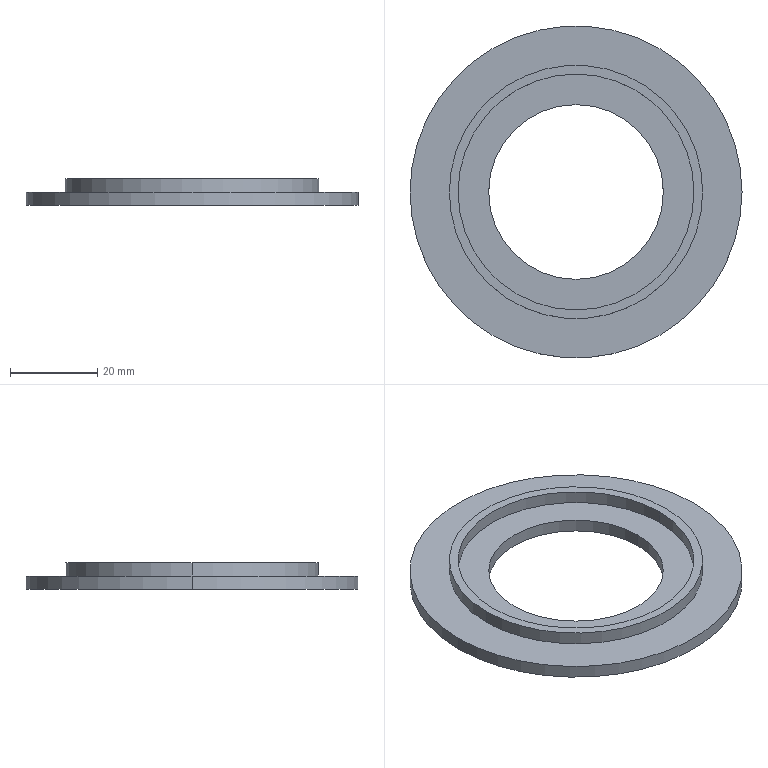Part | STEP file | outer seal | 1 solid | 12 faces | box 76 x 76 x 6 mm | volume 10895 mm3 | cylinder 8 | plane 4 | commonest cylinder face diameters 40 x2 54 x2 58 x2 76 x2
STEP:
#1=CARTESIAN_POINT('',(-20.,0.,0.));
#2=VERTEX_POINT('',#1);
#3=CARTESIAN_POINT('',(20.,0.,0.));
#4=VERTEX_POINT('',#3);
#5=CARTESIAN_POINT('',(0.,0.,0.));
#6=DIRECTION('',(0.,0.,1.));
#7=DIRECTION('',(1.,0.,0.));
#8=AXIS2_PLACEMENT_3D('',#5,#6,#7);
#9=CIRCLE('',#8,20.);
#10=EDGE_CURVE('',#2,#4,#9,.T.);
#11=ORIENTED_EDGE('',*,*,#10,.F.);
#12=CARTESIAN_POINT('',(-20.,0.,3.));
#13=VERTEX_POINT('',#12);
#14=CARTESIAN_POINT('',(-20.,0.,0.));
#15=DIRECTION('',(0.,0.,1.));
#16=VECTOR('',#15,1000.);
#17=LINE('',#14,#16);
#18=EDGE_CURVE('',#2,#13,#17,.T.);
#19=ORIENTED_EDGE('',*,*,#18,.T.);
#20=CARTESIAN_POINT('',(20.,0.,3.));
#21=VERTEX_POINT('',#20);
#22=CARTESIAN_POINT('',(0.,0.,3.));
#23=DIRECTION('',(0.,0.,1.));
#24=DIRECTION('',(1.,0.,0.));
#25=AXIS2_PLACEMENT_3D('',#22,#23,#24);
#26=CIRCLE('',#25,20.);
#27=EDGE_CURVE('',#13,#21,#26,.T.);
#28=ORIENTED_EDGE('',*,*,#27,.T.);
#29=CARTESIAN_POINT('',(20.,0.,0.));
#30=DIRECTION('',(0.,0.,1.));
#31=VECTOR('',#30,1000.);
#32=LINE('',#29,#31);
#33=EDGE_CURVE('',#4,#21,#32,.T.);
#34=ORIENTED_EDGE('',*,*,#33,.F.);
#35=EDGE_LOOP('',(#11,#19,#28,#34));
#36=FACE_OUTER_BOUND('',#35,.T.);
#37=CARTESIAN_POINT('',(0.,0.,0.));
#38=DIRECTION('',(0.,0.,1.));
#39=DIRECTION('',(1.,0.,0.));
#40=AXIS2_PLACEMENT_3D('',#37,#38,#39);
#41=CYLINDRICAL_SURFACE('',#40,20.);
#42=ADVANCED_FACE('',(#36),#41,.F.);
#43=CARTESIAN_POINT('',(-27.,0.,6.));
#44=VERTEX_POINT('',#43);
#45=CARTESIAN_POINT('',(27.,0.,6.));
#46=VERTEX_POINT('',#45);
#47=CARTESIAN_POINT('',(0.,0.,6.));
#48=DIRECTION('',(0.,0.,1.));
#49=DIRECTION('',(1.,0.,0.));
#50=AXIS2_PLACEMENT_3D('',#47,#48,#49);
#51=CIRCLE('',#50,27.);
#52=EDGE_CURVE('',#44,#46,#51,.T.);
#53=ORIENTED_EDGE('',*,*,#52,.T.);
#54=CARTESIAN_POINT('',(27.,0.,3.));
#55=VERTEX_POINT('',#54);
#56=CARTESIAN_POINT('',(27.,0.,6.));
#57=DIRECTION('',(0.,0.,-1.));
#58=VECTOR('',#57,1000.);
#59=LINE('',#56,#58);
#60=EDGE_CURVE('',#46,#55,#59,.T.);
#61=ORIENTED_EDGE('',*,*,#60,.T.);
#62=CARTESIAN_POINT('',(-27.,0.,3.));
#63=VERTEX_POINT('',#62);
#64=CARTESIAN_POINT('',(0.,0.,3.));
#65=DIRECTION('',(0.,0.,-1.));
#66=DIRECTION('',(1.,0.,0.));
#67=AXIS2_PLACEMENT_3D('',#64,#65,#66);
#68=CIRCLE('',#67,27.);
#69=EDGE_CURVE('',#55,#63,#68,.T.);
#70=ORIENTED_EDGE('',*,*,#69,.T.);
#71=CARTESIAN_POINT('',(-27.,0.,6.));
#72=DIRECTION('',(0.,0.,-1.));
#73=VECTOR('',#72,1000.);
#74=LINE('',#71,#73);
#75=EDGE_CURVE('',#44,#63,#74,.T.);
#76=ORIENTED_EDGE('',*,*,#75,.F.);
#77=EDGE_LOOP('',(#53,#61,#70,#76));
#78=FACE_OUTER_BOUND('',#77,.T.);
#79=CARTESIAN_POINT('',(0.,0.,6.));
#80=DIRECTION('',(0.,0.,-1.));
#81=DIRECTION('',(-1.,0.,0.));
#82=AXIS2_PLACEMENT_3D('',#79,#80,#81);
#83=CYLINDRICAL_SURFACE('',#82,27.);
#84=ADVANCED_FACE('',(#78),#83,.F.);
#85=CARTESIAN_POINT('',(29.,0.,6.));
#86=VERTEX_POINT('',#85);
#87=CARTESIAN_POINT('',(-29.,0.,6.));
#88=VERTEX_POINT('',#87);
#89=CARTESIAN_POINT('',(0.,0.,6.));
#90=DIRECTION('',(0.,0.,1.));
#91=DIRECTION('',(1.,0.,0.));
#92=AXIS2_PLACEMENT_3D('',#89,#90,#91);
#93=CIRCLE('',#92,29.);
#94=EDGE_CURVE('',#86,#88,#93,.T.);
#95=ORIENTED_EDGE('',*,*,#94,.F.);
#96=CARTESIAN_POINT('',(29.,0.,3.));
#97=VERTEX_POINT('',#96);
#98=CARTESIAN_POINT('',(29.,0.,6.));
#99=DIRECTION('',(0.,0.,-1.));
#100=VECTOR('',#99,1000.);
#101=LINE('',#98,#100);
#102=EDGE_CURVE('',#86,#97,#101,.T.);
#103=ORIENTED_EDGE('',*,*,#102,.T.);
#104=CARTESIAN_POINT('',(-29.,0.,3.));
#105=VERTEX_POINT('',#104);
#106=CARTESIAN_POINT('',(0.,0.,3.));
#107=DIRECTION('',(0.,0.,1.));
#108=DIRECTION('',(1.,0.,0.));
#109=AXIS2_PLACEMENT_3D('',#106,#107,#108);
#110=CIRCLE('',#109,29.);
#111=EDGE_CURVE('',#97,#105,#110,.T.);
#112=ORIENTED_EDGE('',*,*,#111,.T.);
#113=CARTESIAN_POINT('',(-29.,0.,6.));
#114=DIRECTION('',(0.,0.,-1.));
#115=VECTOR('',#114,1000.);
#116=LINE('',#113,#115);
#117=EDGE_CURVE('',#88,#105,#116,.T.);
#118=ORIENTED_EDGE('',*,*,#117,.F.);
#119=EDGE_LOOP('',(#95,#103,#112,#118));
#120=FACE_OUTER_BOUND('',#119,.T.);
#121=CARTESIAN_POINT('',(0.,0.,6.));
#122=DIRECTION('',(0.,0.,-1.));
#123=DIRECTION('',(-1.,0.,0.));
#124=AXIS2_PLACEMENT_3D('',#121,#122,#123);
#125=CYLINDRICAL_SURFACE('',#124,29.);
#126=ADVANCED_FACE('',(#120),#125,.T.);
#127=CARTESIAN_POINT('',(38.,0.,3.));
#128=VERTEX_POINT('',#127);
#129=CARTESIAN_POINT('',(-38.,0.,3.));
#130=VERTEX_POINT('',#129);
#131=CARTESIAN_POINT('',(0.,0.,3.));
#132=DIRECTION('',(0.,0.,1.));
#133=DIRECTION('',(1.,0.,0.));
#134=AXIS2_PLACEMENT_3D('',#131,#132,#133);
#135=CIRCLE('',#134,38.);
#136=EDGE_CURVE('',#128,#130,#135,.T.);
#137=ORIENTED_EDGE('',*,*,#136,.F.);
#138=CARTESIAN_POINT('',(38.,0.,0.));
#139=VERTEX_POINT('',#138);
#140=CARTESIAN_POINT('',(38.,0.,3.));
#141=DIRECTION('',(0.,0.,-1.));
#142=VECTOR('',#141,1000.);
#143=LINE('',#140,#142);
#144=EDGE_CURVE('',#128,#139,#143,.T.);
#145=ORIENTED_EDGE('',*,*,#144,.T.);
#146=CARTESIAN_POINT('',(-38.,0.,0.));
#147=VERTEX_POINT('',#146);
#148=CARTESIAN_POINT('',(0.,0.,0.));
#149=DIRECTION('',(0.,0.,1.));
#150=DIRECTION('',(1.,0.,0.));
#151=AXIS2_PLACEMENT_3D('',#148,#149,#150);
#152=CIRCLE('',#151,38.);
#153=EDGE_CURVE('',#139,#147,#152,.T.);
#154=ORIENTED_EDGE('',*,*,#153,.T.);
#155=CARTESIAN_POINT('',(-38.,0.,3.));
#156=DIRECTION('',(0.,0.,-1.));
#157=VECTOR('',#156,1000.);
#158=LINE('',#155,#157);
#159=EDGE_CURVE('',#130,#147,#158,.T.);
#160=ORIENTED_EDGE('',*,*,#159,.F.);
#161=EDGE_LOOP('',(#137,#145,#154,#160));
#162=FACE_OUTER_BOUND('',#161,.T.);
#163=CARTESIAN_POINT('',(0.,0.,3.));
#164=DIRECTION('',(0.,0.,-1.));
#165=DIRECTION('',(-1.,0.,0.));
#166=AXIS2_PLACEMENT_3D('',#163,#164,#165);
#167=CYLINDRICAL_SURFACE('',#166,38.);
#168=ADVANCED_FACE('',(#162),#167,.T.);
#169=ORIENTED_EDGE('',*,*,#144,.F.);
#170=CARTESIAN_POINT('',(0.,0.,3.));
#171=DIRECTION('',(0.,0.,1.));
#172=DIRECTION('',(1.,0.,0.));
#173=AXIS2_PLACEMENT_3D('',#170,#171,#172);
#174=CIRCLE('',#173,38.);
#175=EDGE_CURVE('',#130,#128,#174,.T.);
#176=ORIENTED_EDGE('',*,*,#175,.F.);
#177=ORIENTED_EDGE('',*,*,#159,.T.);
#178=CARTESIAN_POINT('',(0.,0.,0.));
#179=DIRECTION('',(0.,0.,1.));
#180=DIRECTION('',(1.,0.,0.));
#181=AXIS2_PLACEMENT_3D('',#178,#179,#180);
#182=CIRCLE('',#181,38.);
#183=EDGE_CURVE('',#147,#139,#182,.T.);
#184=ORIENTED_EDGE('',*,*,#183,.T.);
#185=EDGE_LOOP('',(#169,#176,#177,#184));
#186=FACE_OUTER_BOUND('',#185,.T.);
#187=CARTESIAN_POINT('',(0.,0.,3.));
#188=DIRECTION('',(0.,0.,-1.));
#189=DIRECTION('',(-1.,0.,0.));
#190=AXIS2_PLACEMENT_3D('',#187,#188,#189);
#191=CYLINDRICAL_SURFACE('',#190,38.);
#192=ADVANCED_FACE('',(#186),#191,.T.);
#193=CARTESIAN_POINT('',(0.,0.,3.));
#194=DIRECTION('',(0.,0.,1.));
#195=DIRECTION('',(1.,0.,0.));
#196=AXIS2_PLACEMENT_3D('',#193,#194,#195);
#197=CIRCLE('',#196,29.);
#198=EDGE_CURVE('',#105,#97,#197,.T.);
#199=ORIENTED_EDGE('',*,*,#198,.F.);
#200=ORIENTED_EDGE('',*,*,#111,.F.);
#201=EDGE_LOOP('',(#199,#200));
#202=FACE_BOUND('',#201,.T.);
#203=ORIENTED_EDGE('',*,*,#175,.T.);
#204=ORIENTED_EDGE('',*,*,#136,.T.);
#205=EDGE_LOOP('',(#203,#204));
#206=FACE_OUTER_BOUND('',#205,.T.);
#207=CARTESIAN_POINT('',(0.,0.,3.));
#208=DIRECTION('',(0.,0.,1.));
#209=DIRECTION('',(1.,0.,0.));
#210=AXIS2_PLACEMENT_3D('',#207,#208,#209);
#211=PLANE('',#210);
#212=ADVANCED_FACE('',(#202,#206),#211,.T.);
#213=CARTESIAN_POINT('',(0.,0.,0.));
#214=DIRECTION('',(0.,0.,1.));
#215=DIRECTION('',(1.,0.,0.));
#216=AXIS2_PLACEMENT_3D('',#213,#214,#215);
#217=CIRCLE('',#216,20.);
#218=EDGE_CURVE('',#4,#2,#217,.T.);
#219=ORIENTED_EDGE('',*,*,#218,.T.);
#220=ORIENTED_EDGE('',*,*,#10,.T.);
#221=EDGE_LOOP('',(#219,#220));
#222=FACE_BOUND('',#221,.T.);
#223=ORIENTED_EDGE('',*,*,#183,.F.);
#224=ORIENTED_EDGE('',*,*,#153,.F.);
#225=EDGE_LOOP('',(#223,#224));
#226=FACE_OUTER_BOUND('',#225,.T.);
#227=CARTESIAN_POINT('',(0.,0.,0.));
#228=DIRECTION('',(0.,0.,1.));
#229=DIRECTION('',(1.,0.,0.));
#230=AXIS2_PLACEMENT_3D('',#227,#228,#229);
#231=PLANE('',#230);
#232=ADVANCED_FACE('',(#222,#226),#231,.F.);
#233=CARTESIAN_POINT('',(0.,0.,6.));
#234=DIRECTION('',(0.,0.,1.));
#235=DIRECTION('',(1.,0.,0.));
#236=AXIS2_PLACEMENT_3D('',#233,#234,#235);
#237=CIRCLE('',#236,29.);
#238=EDGE_CURVE('',#88,#86,#237,.T.);
#239=ORIENTED_EDGE('',*,*,#238,.T.);
#240=ORIENTED_EDGE('',*,*,#94,.T.);
#241=EDGE_LOOP('',(#239,#240));
#242=FACE_OUTER_BOUND('',#241,.T.);
#243=ORIENTED_EDGE('',*,*,#52,.F.);
#244=CARTESIAN_POINT('',(0.,0.,6.));
#245=DIRECTION('',(0.,0.,1.));
#246=DIRECTION('',(1.,0.,0.));
#247=AXIS2_PLACEMENT_3D('',#244,#245,#246);
#248=CIRCLE('',#247,27.);
#249=EDGE_CURVE('',#46,#44,#248,.T.);
#250=ORIENTED_EDGE('',*,*,#249,.F.);
#251=EDGE_LOOP('',(#243,#250));
#252=FACE_BOUND('',#251,.T.);
#253=CARTESIAN_POINT('',(0.,0.,6.));
#254=DIRECTION('',(0.,0.,1.));
#255=DIRECTION('',(1.,0.,0.));
#256=AXIS2_PLACEMENT_3D('',#253,#254,#255);
#257=PLANE('',#256);
#258=ADVANCED_FACE('',(#242,#252),#257,.T.);
#259=ORIENTED_EDGE('',*,*,#102,.F.);
#260=ORIENTED_EDGE('',*,*,#238,.F.);
#261=ORIENTED_EDGE('',*,*,#117,.T.);
#262=ORIENTED_EDGE('',*,*,#198,.T.);
#263=EDGE_LOOP('',(#259,#260,#261,#262));
#264=FACE_OUTER_BOUND('',#263,.T.);
#265=CARTESIAN_POINT('',(0.,0.,6.));
#266=DIRECTION('',(0.,0.,-1.));
#267=DIRECTION('',(-1.,0.,0.));
#268=AXIS2_PLACEMENT_3D('',#265,#266,#267);
#269=CYLINDRICAL_SURFACE('',#268,29.);
#270=ADVANCED_FACE('',(#264),#269,.T.);
#271=ORIENTED_EDGE('',*,*,#60,.F.);
#272=ORIENTED_EDGE('',*,*,#249,.T.);
#273=ORIENTED_EDGE('',*,*,#75,.T.);
#274=CARTESIAN_POINT('',(0.,0.,3.));
#275=DIRECTION('',(0.,0.,-1.));
#276=DIRECTION('',(1.,0.,0.));
#277=AXIS2_PLACEMENT_3D('',#274,#275,#276);
#278=CIRCLE('',#277,27.);
#279=EDGE_CURVE('',#63,#55,#278,.T.);
#280=ORIENTED_EDGE('',*,*,#279,.T.);
#281=EDGE_LOOP('',(#271,#272,#273,#280));
#282=FACE_OUTER_BOUND('',#281,.T.);
#283=CARTESIAN_POINT('',(0.,0.,6.));
#284=DIRECTION('',(0.,0.,-1.));
#285=DIRECTION('',(-1.,0.,0.));
#286=AXIS2_PLACEMENT_3D('',#283,#284,#285);
#287=CYLINDRICAL_SURFACE('',#286,27.);
#288=ADVANCED_FACE('',(#282),#287,.F.);
#289=CARTESIAN_POINT('',(0.,0.,3.));
#290=DIRECTION('',(0.,0.,1.));
#291=DIRECTION('',(1.,0.,0.));
#292=AXIS2_PLACEMENT_3D('',#289,#290,#291);
#293=CIRCLE('',#292,20.);
#294=EDGE_CURVE('',#21,#13,#293,.T.);
#295=ORIENTED_EDGE('',*,*,#294,.F.);
#296=ORIENTED_EDGE('',*,*,#27,.F.);
#297=EDGE_LOOP('',(#295,#296));
#298=FACE_BOUND('',#297,.T.);
#299=ORIENTED_EDGE('',*,*,#279,.F.);
#300=ORIENTED_EDGE('',*,*,#69,.F.);
#301=EDGE_LOOP('',(#299,#300));
#302=FACE_OUTER_BOUND('',#301,.T.);
#303=CARTESIAN_POINT('',(0.,0.,3.));
#304=DIRECTION('',(0.,0.,1.));
#305=DIRECTION('',(1.,0.,0.));
#306=AXIS2_PLACEMENT_3D('',#303,#304,#305);
#307=PLANE('',#306);
#308=ADVANCED_FACE('',(#298,#302),#307,.T.);
#309=ORIENTED_EDGE('',*,*,#18,.F.);
#310=ORIENTED_EDGE('',*,*,#218,.F.);
#311=ORIENTED_EDGE('',*,*,#33,.T.);
#312=ORIENTED_EDGE('',*,*,#294,.T.);
#313=EDGE_LOOP('',(#309,#310,#311,#312));
#314=FACE_OUTER_BOUND('',#313,.T.);
#315=CARTESIAN_POINT('',(0.,0.,0.));
#316=DIRECTION('',(0.,0.,1.));
#317=DIRECTION('',(1.,0.,0.));
#318=AXIS2_PLACEMENT_3D('',#315,#316,#317);
#319=CYLINDRICAL_SURFACE('',#318,20.);
#320=ADVANCED_FACE('',(#314),#319,.F.);
#321=CLOSED_SHELL('',(#42,#84,#126,#168,#192,#212,#232,#258,#270,#288,#308,#320));
#322=MANIFOLD_SOLID_BREP('',#321);
#323=CARTESIAN_POINT('',(0.,0.,0.));
#324=DIRECTION('',(0.,0.,1.));
#325=DIRECTION('',(1.,0.,0.));
#326=AXIS2_PLACEMENT_3D('',#323,#324,#325);
#327=(LENGTH_UNIT()NAMED_UNIT(*)SI_UNIT(.MILLI.,.METRE.));
#328=UNCERTAINTY_MEASURE_WITH_UNIT(LENGTH_MEASURE(0.00001),#327,'','');
#329=(NAMED_UNIT(*)PLANE_ANGLE_UNIT()SI_UNIT($,.RADIAN.));
#330=(NAMED_UNIT(*)SI_UNIT($,.STERADIAN.)SOLID_ANGLE_UNIT());
#331=(GEOMETRIC_REPRESENTATION_CONTEXT(3)GLOBAL_UNCERTAINTY_ASSIGNED_CONTEXT((#328))GLOBAL_UNIT_ASSIGNED_CONTEXT((#327,#329,#330))REPRESENTATION_CONTEXT('',''));
#332=ADVANCED_BREP_SHAPE_REPRESENTATION('',(#322,#326),#331);